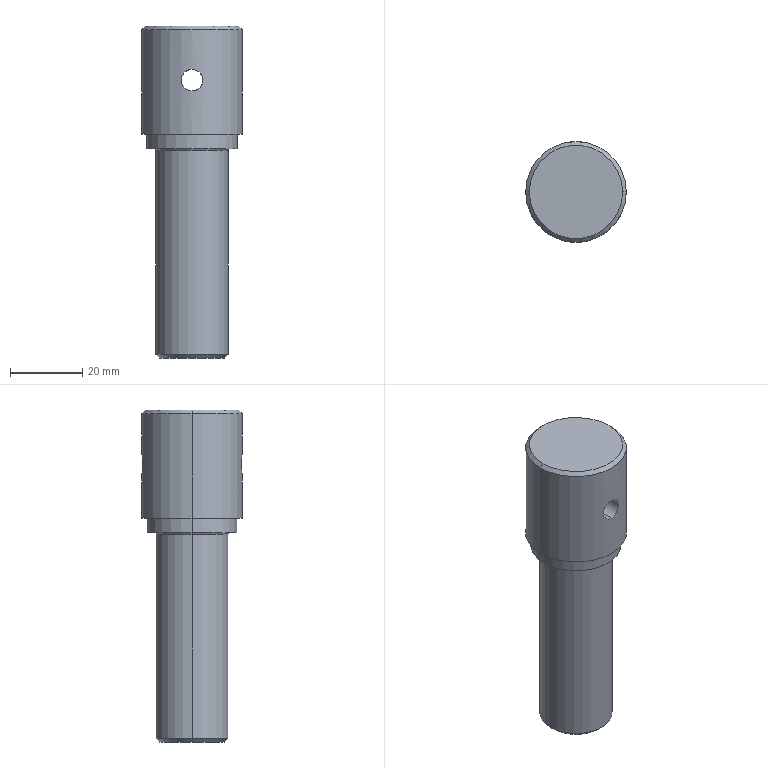Part | SolidWorks | features ICE 3, Chamfer 1, Extrusion 1, Fillet 1 | 1 solid | 18 faces | box 27.9 x 27.9 x 92 mm | volume 37672 mm3 | cylinder 8 | cone 4 | plane 4 | torus 2 | commonest cylinder face diameters 6 x2 20 x2 25 x2 27.9 x2
STEP:
#1=CARTESIAN_POINT('',(0.,-13.95,74.));
#2=VERTEX_POINT('',#1);
#3=CARTESIAN_POINT('',(0.,-13.95,80.));
#4=VERTEX_POINT('',#3);
#5=CARTESIAN_POINT('',(0.,-13.95,74.));
#6=CARTESIAN_POINT('',(-0.3921,-13.95,74.));
#7=CARTESIAN_POINT('',(-0.788,-13.932,74.079));
#8=CARTESIAN_POINT('',(-1.33,-13.888,74.304));
#9=CARTESIAN_POINT('',(-1.505,-13.87,74.397));
#10=CARTESIAN_POINT('',(-1.831,-13.83,74.616));
#11=CARTESIAN_POINT('',(-1.982,-13.809,74.739));
#12=CARTESIAN_POINT('',(-2.259,-13.767,75.016));
#13=CARTESIAN_POINT('',(-2.385,-13.745,75.17));
#14=CARTESIAN_POINT('',(-2.602,-13.706,75.494));
#15=CARTESIAN_POINT('',(-2.694,-13.688,75.666));
#16=CARTESIAN_POINT('',(-2.922,-13.642,76.212));
#17=CARTESIAN_POINT('',(-3.,-13.624,76.603));
#18=CARTESIAN_POINT('',(-3.,-13.624,77.197));
#19=CARTESIAN_POINT('',(-2.981,-13.628,77.392));
#20=CARTESIAN_POINT('',(-2.904,-13.644,77.776));
#21=CARTESIAN_POINT('',(-2.846,-13.657,77.968));
#22=CARTESIAN_POINT('',(-2.696,-13.687,78.33));
#23=CARTESIAN_POINT('',(-2.604,-13.705,78.502));
#24=CARTESIAN_POINT('',(-2.386,-13.745,78.829));
#25=CARTESIAN_POINT('',(-2.26,-13.766,78.982));
#26=CARTESIAN_POINT('',(-1.847,-13.83,79.396));
#27=CARTESIAN_POINT('',(-1.514,-13.872,79.619));
#28=CARTESIAN_POINT('',(-0.9725,-13.917,79.845));
#29=CARTESIAN_POINT('',(-0.7819,-13.929,79.903));
#30=CARTESIAN_POINT('',(-0.3949,-13.946,79.98));
#31=CARTESIAN_POINT('',(-0.1988,-13.95,80.));
#32=CARTESIAN_POINT('',(0.,-13.95,80.));
#33=B_SPLINE_CURVE_WITH_KNOTS('',3,(#5,#6,#7,#8,#9,#10,#11,#12,#13,#14,#15,#16,#17,#18,#19,#20,#21,#22,#23,#24,#25,#26,#27,#28,#29,#30,#31,#32),.UNSPECIFIED.,.F.,.F.,(4,2,2,2,2,2,2,2,2,2,2,2,2,4),(0.009407,0.01058,0.01117,0.01176,0.01235,0.01293,0.01411,0.0147,0.01528,0.01587,0.01646,0.01764,0.01822,0.01881),.UNSPECIFIED.);
#34=EDGE_CURVE('',#2,#4,#33,.T.);
#35=ORIENTED_EDGE('',*,*,#34,.F.);
#36=CARTESIAN_POINT('',(0.,13.95,74.));
#37=VERTEX_POINT('',#36);
#38=CARTESIAN_POINT('',(0.,-15.,74.));
#39=DIRECTION('',(0.,1.,0.));
#40=VECTOR('',#39,1000.);
#41=LINE('',#38,#40);
#42=EDGE_CURVE('',#2,#37,#41,.T.);
#43=ORIENTED_EDGE('',*,*,#42,.T.);
#44=CARTESIAN_POINT('',(0.,13.95,80.));
#45=VERTEX_POINT('',#44);
#46=CARTESIAN_POINT('',(0.,13.95,80.));
#47=CARTESIAN_POINT('',(-0.1988,13.95,80.));
#48=CARTESIAN_POINT('',(-0.3942,13.946,79.98));
#49=CARTESIAN_POINT('',(-0.7785,13.93,79.904));
#50=CARTESIAN_POINT('',(-0.9694,13.917,79.846));
#51=CARTESIAN_POINT('',(-1.332,13.887,79.695));
#52=CARTESIAN_POINT('',(-1.505,13.87,79.603));
#53=CARTESIAN_POINT('',(-1.83,13.83,79.385));
#54=CARTESIAN_POINT('',(-1.984,13.809,79.259));
#55=CARTESIAN_POINT('',(-2.26,13.766,78.983));
#56=CARTESIAN_POINT('',(-2.384,13.745,78.832));
#57=CARTESIAN_POINT('',(-2.603,13.705,78.504));
#58=CARTESIAN_POINT('',(-2.696,13.687,78.331));
#59=CARTESIAN_POINT('',(-2.846,13.657,77.97));
#60=CARTESIAN_POINT('',(-2.904,13.645,77.78));
#61=CARTESIAN_POINT('',(-2.981,13.628,77.393));
#62=CARTESIAN_POINT('',(-3.,13.624,77.198));
#63=CARTESIAN_POINT('',(-3.,13.624,76.805));
#64=CARTESIAN_POINT('',(-2.98,13.628,76.605));
#65=CARTESIAN_POINT('',(-2.904,13.645,76.22));
#66=CARTESIAN_POINT('',(-2.847,13.657,76.033));
#67=CARTESIAN_POINT('',(-2.696,13.687,75.669));
#68=CARTESIAN_POINT('',(-2.602,13.706,75.494));
#69=CARTESIAN_POINT('',(-2.385,13.745,75.17));
#70=CARTESIAN_POINT('',(-2.26,13.766,75.018));
#71=CARTESIAN_POINT('',(-1.982,13.809,74.739));
#72=CARTESIAN_POINT('',(-1.831,13.83,74.615));
#73=CARTESIAN_POINT('',(-1.506,13.869,74.398));
#74=CARTESIAN_POINT('',(-1.331,13.888,74.304));
#75=CARTESIAN_POINT('',(-0.9682,13.918,74.154));
#76=CARTESIAN_POINT('',(-0.7811,13.929,74.097));
#77=CARTESIAN_POINT('',(-0.3953,13.946,74.02));
#78=CARTESIAN_POINT('',(-0.1961,13.95,74.));
#79=CARTESIAN_POINT('',(0.,13.95,74.));
#80=B_SPLINE_CURVE_WITH_KNOTS('',3,(#46,#47,#48,#49,#50,#51,#52,#53,#54,#55,#56,#57,#58,#59,#60,#61,#62,#63,#64,#65,#66,#67,#68,#69,#70,#71,#72,#73,#74,#75,#76,#77,#78,#79),.UNSPECIFIED.,.F.,.F.,(4,2,2,2,2,2,2,2,2,2,2,2,2,2,2,2,4),(0.,0.0005879,0.001176,0.001764,0.002352,0.00294,0.003528,0.004116,0.004703,0.005291,0.005879,0.006467,0.007055,0.007643,0.008231,0.008819,0.009407),.UNSPECIFIED.);
#81=EDGE_CURVE('',#45,#37,#80,.T.);
#82=ORIENTED_EDGE('',*,*,#81,.F.);
#83=CARTESIAN_POINT('',(0.,-15.,80.));
#84=DIRECTION('',(0.,1.,0.));
#85=VECTOR('',#84,1000.);
#86=LINE('',#83,#85);
#87=EDGE_CURVE('',#4,#45,#86,.T.);
#88=ORIENTED_EDGE('',*,*,#87,.F.);
#89=EDGE_LOOP('',(#35,#43,#82,#88));
#90=FACE_OUTER_BOUND('',#89,.T.);
#91=CARTESIAN_POINT('',(0.,-15.,77.));
#92=DIRECTION('',(0.,1.,0.));
#93=DIRECTION('',(0.,0.,1.));
#94=AXIS2_PLACEMENT_3D('',#91,#92,#93);
#95=CYLINDRICAL_SURFACE('',#94,3.);
#96=ADVANCED_FACE('',(#90),#95,.F.);
#97=CARTESIAN_POINT('',(-10.5,0.,58.));
#98=VERTEX_POINT('',#97);
#99=CARTESIAN_POINT('',(10.5,0.,58.));
#100=VERTEX_POINT('',#99);
#101=CARTESIAN_POINT('',(0.,0.,58.));
#102=DIRECTION('',(0.,0.,1.));
#103=DIRECTION('',(1.,0.,0.));
#104=AXIS2_PLACEMENT_3D('',#101,#102,#103);
#105=CIRCLE('',#104,10.5);
#106=EDGE_CURVE('',#98,#100,#105,.T.);
#107=ORIENTED_EDGE('',*,*,#106,.F.);
#108=CARTESIAN_POINT('',(-10.,0.,57.5));
#109=VERTEX_POINT('',#108);
#110=CARTESIAN_POINT('',(-10.5,0.,57.5));
#111=DIRECTION('',(0.,1.,0.));
#112=DIRECTION('',(-1.,0.,0.));
#113=AXIS2_PLACEMENT_3D('',#110,#111,#112);
#114=CIRCLE('',#113,0.5);
#115=EDGE_CURVE('',#98,#109,#114,.T.);
#116=ORIENTED_EDGE('',*,*,#115,.T.);
#117=CARTESIAN_POINT('',(10.,0.,57.5));
#118=VERTEX_POINT('',#117);
#119=CARTESIAN_POINT('',(0.,0.,57.5));
#120=DIRECTION('',(0.,0.,-1.));
#121=DIRECTION('',(1.,0.,0.));
#122=AXIS2_PLACEMENT_3D('',#119,#120,#121);
#123=CIRCLE('',#122,10.);
#124=EDGE_CURVE('',#118,#109,#123,.T.);
#125=ORIENTED_EDGE('',*,*,#124,.F.);
#126=CARTESIAN_POINT('',(10.5,0.,57.5));
#127=DIRECTION('',(0.,-1.,0.));
#128=DIRECTION('',(0.,0.,-1.));
#129=AXIS2_PLACEMENT_3D('',#126,#127,#128);
#130=CIRCLE('',#129,0.5);
#131=EDGE_CURVE('',#100,#118,#130,.T.);
#132=ORIENTED_EDGE('',*,*,#131,.F.);
#133=EDGE_LOOP('',(#107,#116,#125,#132));
#134=FACE_OUTER_BOUND('',#133,.T.);
#135=CARTESIAN_POINT('',(0.,0.,57.5));
#136=DIRECTION('',(0.,0.,1.));
#137=DIRECTION('',(1.,0.,0.));
#138=AXIS2_PLACEMENT_3D('',#135,#136,#137);
#139=TOROIDAL_SURFACE('',#138,10.5,0.5);
#140=ADVANCED_FACE('',(#134),#139,.F.);
#141=CARTESIAN_POINT('',(12.95,0.,92.));
#142=VERTEX_POINT('',#141);
#143=CARTESIAN_POINT('',(-12.95,0.,92.));
#144=VERTEX_POINT('',#143);
#145=CARTESIAN_POINT('',(0.,0.,92.));
#146=DIRECTION('',(0.,0.,1.));
#147=DIRECTION('',(1.,0.,0.));
#148=AXIS2_PLACEMENT_3D('',#145,#146,#147);
#149=CIRCLE('',#148,12.95);
#150=EDGE_CURVE('',#142,#144,#149,.T.);
#151=ORIENTED_EDGE('',*,*,#150,.F.);
#152=CARTESIAN_POINT('',(13.95,0.,91.));
#153=VERTEX_POINT('',#152);
#154=CARTESIAN_POINT('',(12.95,0.,92.));
#155=DIRECTION('',(0.7071,0.,-0.7071));
#156=VECTOR('',#155,1000.);
#157=LINE('',#154,#156);
#158=EDGE_CURVE('',#142,#153,#157,.T.);
#159=ORIENTED_EDGE('',*,*,#158,.T.);
#160=CARTESIAN_POINT('',(-13.95,0.,91.));
#161=VERTEX_POINT('',#160);
#162=CARTESIAN_POINT('',(0.,0.,91.));
#163=DIRECTION('',(0.,0.,-1.));
#164=DIRECTION('',(1.,0.,0.));
#165=AXIS2_PLACEMENT_3D('',#162,#163,#164);
#166=CIRCLE('',#165,13.95);
#167=EDGE_CURVE('',#161,#153,#166,.T.);
#168=ORIENTED_EDGE('',*,*,#167,.F.);
#169=CARTESIAN_POINT('',(-12.95,0.,92.));
#170=DIRECTION('',(-0.7071,0.,-0.7071));
#171=VECTOR('',#170,1000.);
#172=LINE('',#169,#171);
#173=EDGE_CURVE('',#144,#161,#172,.T.);
#174=ORIENTED_EDGE('',*,*,#173,.F.);
#175=EDGE_LOOP('',(#151,#159,#168,#174));
#176=FACE_OUTER_BOUND('',#175,.T.);
#177=CARTESIAN_POINT('',(0.,0.,92.));
#178=DIRECTION('',(0.,0.,-1.));
#179=DIRECTION('',(-1.,0.,0.));
#180=AXIS2_PLACEMENT_3D('',#177,#178,#179);
#181=CONICAL_SURFACE('',#180,12.95,0.7854);
#182=ADVANCED_FACE('',(#176),#181,.T.);
#183=CARTESIAN_POINT('',(-9.,0.,0.));
#184=VERTEX_POINT('',#183);
#185=CARTESIAN_POINT('',(9.,0.,0.));
#186=VERTEX_POINT('',#185);
#187=CARTESIAN_POINT('',(0.,0.,0.));
#188=DIRECTION('',(0.,0.,-1.));
#189=DIRECTION('',(1.,0.,0.));
#190=AXIS2_PLACEMENT_3D('',#187,#188,#189);
#191=CIRCLE('',#190,9.);
#192=EDGE_CURVE('',#184,#186,#191,.T.);
#193=ORIENTED_EDGE('',*,*,#192,.F.);
#194=CARTESIAN_POINT('',(-10.,0.,1.));
#195=VERTEX_POINT('',#194);
#196=CARTESIAN_POINT('',(-10.,0.,1.));
#197=DIRECTION('',(-0.7071,0.,0.7071));
#198=VECTOR('',#197,1000.);
#199=LINE('',#196,#198);
#200=EDGE_CURVE('',#184,#195,#199,.T.);
#201=ORIENTED_EDGE('',*,*,#200,.T.);
#202=CARTESIAN_POINT('',(10.,0.,1.));
#203=VERTEX_POINT('',#202);
#204=CARTESIAN_POINT('',(0.,0.,1.));
#205=DIRECTION('',(0.,0.,1.));
#206=DIRECTION('',(1.,0.,0.));
#207=AXIS2_PLACEMENT_3D('',#204,#205,#206);
#208=CIRCLE('',#207,10.);
#209=EDGE_CURVE('',#203,#195,#208,.T.);
#210=ORIENTED_EDGE('',*,*,#209,.F.);
#211=CARTESIAN_POINT('',(10.,0.,1.));
#212=DIRECTION('',(0.7071,0.,0.7071));
#213=VECTOR('',#212,1000.);
#214=LINE('',#211,#213);
#215=EDGE_CURVE('',#186,#203,#214,.T.);
#216=ORIENTED_EDGE('',*,*,#215,.F.);
#217=EDGE_LOOP('',(#193,#201,#210,#216));
#218=FACE_OUTER_BOUND('',#217,.T.);
#219=CARTESIAN_POINT('',(0.,0.,1.));
#220=DIRECTION('',(0.,0.,1.));
#221=DIRECTION('',(1.,0.,0.));
#222=AXIS2_PLACEMENT_3D('',#219,#220,#221);
#223=CONICAL_SURFACE('',#222,10.,0.7854);
#224=ADVANCED_FACE('',(#218),#223,.T.);
#225=ORIENTED_EDGE('',*,*,#81,.T.);
#226=CARTESIAN_POINT('',(0.,13.95,74.));
#227=CARTESIAN_POINT('',(0.3921,13.95,74.));
#228=CARTESIAN_POINT('',(0.788,13.932,74.079));
#229=CARTESIAN_POINT('',(1.33,13.888,74.304));
#230=CARTESIAN_POINT('',(1.505,13.87,74.397));
#231=CARTESIAN_POINT('',(1.831,13.83,74.616));
#232=CARTESIAN_POINT('',(1.982,13.809,74.739));
#233=CARTESIAN_POINT('',(2.259,13.767,75.016));
#234=CARTESIAN_POINT('',(2.385,13.745,75.17));
#235=CARTESIAN_POINT('',(2.602,13.706,75.494));
#236=CARTESIAN_POINT('',(2.694,13.688,75.666));
#237=CARTESIAN_POINT('',(2.922,13.642,76.212));
#238=CARTESIAN_POINT('',(3.,13.624,76.603));
#239=CARTESIAN_POINT('',(3.,13.624,77.197));
#240=CARTESIAN_POINT('',(2.981,13.628,77.392));
#241=CARTESIAN_POINT('',(2.904,13.644,77.776));
#242=CARTESIAN_POINT('',(2.846,13.657,77.968));
#243=CARTESIAN_POINT('',(2.696,13.687,78.33));
#244=CARTESIAN_POINT('',(2.604,13.705,78.502));
#245=CARTESIAN_POINT('',(2.386,13.745,78.829));
#246=CARTESIAN_POINT('',(2.26,13.766,78.982));
#247=CARTESIAN_POINT('',(1.847,13.83,79.396));
#248=CARTESIAN_POINT('',(1.514,13.872,79.619));
#249=CARTESIAN_POINT('',(0.9725,13.917,79.845));
#250=CARTESIAN_POINT('',(0.7819,13.929,79.903));
#251=CARTESIAN_POINT('',(0.3949,13.946,79.98));
#252=CARTESIAN_POINT('',(0.1988,13.95,80.));
#253=CARTESIAN_POINT('',(0.,13.95,80.));
#254=B_SPLINE_CURVE_WITH_KNOTS('',3,(#226,#227,#228,#229,#230,#231,#232,#233,#234,#235,#236,#237,#238,#239,#240,#241,#242,#243,#244,#245,#246,#247,#248,#249,#250,#251,#252,#253),.UNSPECIFIED.,.F.,.F.,(4,2,2,2,2,2,2,2,2,2,2,2,2,4),(0.009407,0.01058,0.01117,0.01176,0.01235,0.01293,0.01411,0.0147,0.01528,0.01587,0.01646,0.01764,0.01822,0.01881),.UNSPECIFIED.);
#255=EDGE_CURVE('',#37,#45,#254,.T.);
#256=ORIENTED_EDGE('',*,*,#255,.T.);
#257=EDGE_LOOP('',(#225,#256));
#258=FACE_BOUND('',#257,.T.);
#259=ORIENTED_EDGE('',*,*,#167,.T.);
#260=CARTESIAN_POINT('',(13.95,0.,62.));
#261=VERTEX_POINT('',#260);
#262=CARTESIAN_POINT('',(13.95,0.,92.));
#263=DIRECTION('',(0.,0.,-1.));
#264=VECTOR('',#263,1000.);
#265=LINE('',#262,#264);
#266=EDGE_CURVE('',#153,#261,#265,.T.);
#267=ORIENTED_EDGE('',*,*,#266,.T.);
#268=CARTESIAN_POINT('',(-13.95,0.,62.));
#269=VERTEX_POINT('',#268);
#270=CARTESIAN_POINT('',(0.,0.,62.));
#271=DIRECTION('',(0.,0.,1.));
#272=DIRECTION('',(1.,0.,0.));
#273=AXIS2_PLACEMENT_3D('',#270,#271,#272);
#274=CIRCLE('',#273,13.95);
#275=EDGE_CURVE('',#261,#269,#274,.T.);
#276=ORIENTED_EDGE('',*,*,#275,.T.);
#277=CARTESIAN_POINT('',(-13.95,0.,92.));
#278=DIRECTION('',(0.,0.,-1.));
#279=VECTOR('',#278,1000.);
#280=LINE('',#277,#279);
#281=EDGE_CURVE('',#161,#269,#280,.T.);
#282=ORIENTED_EDGE('',*,*,#281,.F.);
#283=EDGE_LOOP('',(#259,#267,#276,#282));
#284=FACE_OUTER_BOUND('',#283,.T.);
#285=CARTESIAN_POINT('',(0.,0.,92.));
#286=DIRECTION('',(0.,0.,-1.));
#287=DIRECTION('',(-1.,0.,0.));
#288=AXIS2_PLACEMENT_3D('',#285,#286,#287);
#289=CYLINDRICAL_SURFACE('',#288,13.95);
#290=ADVANCED_FACE('',(#258,#284),#289,.T.);
#291=CARTESIAN_POINT('',(12.5,0.,62.));
#292=VERTEX_POINT('',#291);
#293=CARTESIAN_POINT('',(-12.5,0.,62.));
#294=VERTEX_POINT('',#293);
#295=CARTESIAN_POINT('',(0.,0.,62.));
#296=DIRECTION('',(0.,0.,1.));
#297=DIRECTION('',(1.,0.,0.));
#298=AXIS2_PLACEMENT_3D('',#295,#296,#297);
#299=CIRCLE('',#298,12.5);
#300=EDGE_CURVE('',#292,#294,#299,.T.);
#301=ORIENTED_EDGE('',*,*,#300,.F.);
#302=CARTESIAN_POINT('',(12.5,0.,58.));
#303=VERTEX_POINT('',#302);
#304=CARTESIAN_POINT('',(12.5,0.,62.));
#305=DIRECTION('',(0.,0.,-1.));
#306=VECTOR('',#305,1000.);
#307=LINE('',#304,#306);
#308=EDGE_CURVE('',#292,#303,#307,.T.);
#309=ORIENTED_EDGE('',*,*,#308,.T.);
#310=CARTESIAN_POINT('',(-12.5,0.,58.));
#311=VERTEX_POINT('',#310);
#312=CARTESIAN_POINT('',(0.,0.,58.));
#313=DIRECTION('',(0.,0.,1.));
#314=DIRECTION('',(1.,0.,0.));
#315=AXIS2_PLACEMENT_3D('',#312,#313,#314);
#316=CIRCLE('',#315,12.5);
#317=EDGE_CURVE('',#303,#311,#316,.T.);
#318=ORIENTED_EDGE('',*,*,#317,.T.);
#319=CARTESIAN_POINT('',(-12.5,0.,62.));
#320=DIRECTION('',(0.,0.,-1.));
#321=VECTOR('',#320,1000.);
#322=LINE('',#319,#321);
#323=EDGE_CURVE('',#294,#311,#322,.T.);
#324=ORIENTED_EDGE('',*,*,#323,.F.);
#325=EDGE_LOOP('',(#301,#309,#318,#324));
#326=FACE_OUTER_BOUND('',#325,.T.);
#327=CARTESIAN_POINT('',(0.,0.,62.));
#328=DIRECTION('',(0.,0.,-1.));
#329=DIRECTION('',(-1.,0.,0.));
#330=AXIS2_PLACEMENT_3D('',#327,#328,#329);
#331=CYLINDRICAL_SURFACE('',#330,12.5);
#332=ADVANCED_FACE('',(#326),#331,.T.);
#333=CARTESIAN_POINT('',(0.,0.,57.5));
#334=DIRECTION('',(0.,0.,-1.));
#335=DIRECTION('',(1.,0.,0.));
#336=AXIS2_PLACEMENT_3D('',#333,#334,#335);
#337=CIRCLE('',#336,10.);
#338=EDGE_CURVE('',#109,#118,#337,.T.);
#339=ORIENTED_EDGE('',*,*,#338,.T.);
#340=CARTESIAN_POINT('',(10.,0.,58.));
#341=DIRECTION('',(0.,0.,-1.));
#342=VECTOR('',#341,1000.);
#343=LINE('',#340,#342);
#344=EDGE_CURVE('',#118,#203,#343,.T.);
#345=ORIENTED_EDGE('',*,*,#344,.T.);
#346=ORIENTED_EDGE('',*,*,#209,.T.);
#347=CARTESIAN_POINT('',(-10.,0.,58.));
#348=DIRECTION('',(0.,0.,-1.));
#349=VECTOR('',#348,1000.);
#350=LINE('',#347,#349);
#351=EDGE_CURVE('',#109,#195,#350,.T.);
#352=ORIENTED_EDGE('',*,*,#351,.F.);
#353=EDGE_LOOP('',(#339,#345,#346,#352));
#354=FACE_OUTER_BOUND('',#353,.T.);
#355=CARTESIAN_POINT('',(0.,0.,58.));
#356=DIRECTION('',(0.,0.,-1.));
#357=DIRECTION('',(-1.,0.,0.));
#358=AXIS2_PLACEMENT_3D('',#355,#356,#357);
#359=CYLINDRICAL_SURFACE('',#358,10.);
#360=ADVANCED_FACE('',(#354),#359,.T.);
#361=ORIENTED_EDGE('',*,*,#344,.F.);
#362=ORIENTED_EDGE('',*,*,#124,.T.);
#363=ORIENTED_EDGE('',*,*,#351,.T.);
#364=CARTESIAN_POINT('',(0.,0.,1.));
#365=DIRECTION('',(0.,0.,1.));
#366=DIRECTION('',(1.,0.,0.));
#367=AXIS2_PLACEMENT_3D('',#364,#365,#366);
#368=CIRCLE('',#367,10.);
#369=EDGE_CURVE('',#195,#203,#368,.T.);
#370=ORIENTED_EDGE('',*,*,#369,.T.);
#371=EDGE_LOOP('',(#361,#362,#363,#370));
#372=FACE_OUTER_BOUND('',#371,.T.);
#373=CARTESIAN_POINT('',(0.,0.,58.));
#374=DIRECTION('',(0.,0.,-1.));
#375=DIRECTION('',(-1.,0.,0.));
#376=AXIS2_PLACEMENT_3D('',#373,#374,#375);
#377=CYLINDRICAL_SURFACE('',#376,10.);
#378=ADVANCED_FACE('',(#372),#377,.T.);
#379=CARTESIAN_POINT('',(0.,0.,0.));
#380=DIRECTION('',(0.,0.,-1.));
#381=DIRECTION('',(1.,0.,0.));
#382=AXIS2_PLACEMENT_3D('',#379,#380,#381);
#383=CIRCLE('',#382,9.);
#384=EDGE_CURVE('',#186,#184,#383,.T.);
#385=ORIENTED_EDGE('',*,*,#384,.T.);
#386=ORIENTED_EDGE('',*,*,#192,.T.);
#387=EDGE_LOOP('',(#385,#386));
#388=FACE_OUTER_BOUND('',#387,.T.);
#389=CARTESIAN_POINT('',(0.,0.,0.));
#390=DIRECTION('',(0.,0.,1.));
#391=DIRECTION('',(1.,0.,0.));
#392=AXIS2_PLACEMENT_3D('',#389,#390,#391);
#393=PLANE('',#392);
#394=ADVANCED_FACE('',(#388),#393,.F.);
#395=ORIENTED_EDGE('',*,*,#308,.F.);
#396=CARTESIAN_POINT('',(0.,0.,62.));
#397=DIRECTION('',(0.,0.,1.));
#398=DIRECTION('',(1.,0.,0.));
#399=AXIS2_PLACEMENT_3D('',#396,#397,#398);
#400=CIRCLE('',#399,12.5);
#401=EDGE_CURVE('',#294,#292,#400,.T.);
#402=ORIENTED_EDGE('',*,*,#401,.F.);
#403=ORIENTED_EDGE('',*,*,#323,.T.);
#404=CARTESIAN_POINT('',(0.,0.,58.));
#405=DIRECTION('',(0.,0.,1.));
#406=DIRECTION('',(1.,0.,0.));
#407=AXIS2_PLACEMENT_3D('',#404,#405,#406);
#408=CIRCLE('',#407,12.5);
#409=EDGE_CURVE('',#311,#303,#408,.T.);
#410=ORIENTED_EDGE('',*,*,#409,.T.);
#411=EDGE_LOOP('',(#395,#402,#403,#410));
#412=FACE_OUTER_BOUND('',#411,.T.);
#413=CARTESIAN_POINT('',(0.,0.,62.));
#414=DIRECTION('',(0.,0.,-1.));
#415=DIRECTION('',(-1.,0.,0.));
#416=AXIS2_PLACEMENT_3D('',#413,#414,#415);
#417=CYLINDRICAL_SURFACE('',#416,12.5);
#418=ADVANCED_FACE('',(#412),#417,.T.);
#419=CARTESIAN_POINT('',(0.,0.,58.));
#420=DIRECTION('',(0.,0.,1.));
#421=DIRECTION('',(1.,0.,0.));
#422=AXIS2_PLACEMENT_3D('',#419,#420,#421);
#423=CIRCLE('',#422,10.5);
#424=EDGE_CURVE('',#100,#98,#423,.T.);
#425=ORIENTED_EDGE('',*,*,#424,.T.);
#426=ORIENTED_EDGE('',*,*,#106,.T.);
#427=EDGE_LOOP('',(#425,#426));
#428=FACE_BOUND('',#427,.T.);
#429=ORIENTED_EDGE('',*,*,#409,.F.);
#430=ORIENTED_EDGE('',*,*,#317,.F.);
#431=EDGE_LOOP('',(#429,#430));
#432=FACE_OUTER_BOUND('',#431,.T.);
#433=CARTESIAN_POINT('',(0.,0.,58.));
#434=DIRECTION('',(0.,0.,1.));
#435=DIRECTION('',(1.,0.,0.));
#436=AXIS2_PLACEMENT_3D('',#433,#434,#435);
#437=PLANE('',#436);
#438=ADVANCED_FACE('',(#428,#432),#437,.F.);
#439=ORIENTED_EDGE('',*,*,#266,.F.);
#440=CARTESIAN_POINT('',(0.,0.,91.));
#441=DIRECTION('',(0.,0.,-1.));
#442=DIRECTION('',(1.,0.,0.));
#443=AXIS2_PLACEMENT_3D('',#440,#441,#442);
#444=CIRCLE('',#443,13.95);
#445=EDGE_CURVE('',#153,#161,#444,.T.);
#446=ORIENTED_EDGE('',*,*,#445,.T.);
#447=ORIENTED_EDGE('',*,*,#281,.T.);
#448=CARTESIAN_POINT('',(0.,0.,62.));
#449=DIRECTION('',(0.,0.,1.));
#450=DIRECTION('',(1.,0.,0.));
#451=AXIS2_PLACEMENT_3D('',#448,#449,#450);
#452=CIRCLE('',#451,13.95);
#453=EDGE_CURVE('',#269,#261,#452,.T.);
#454=ORIENTED_EDGE('',*,*,#453,.T.);
#455=EDGE_LOOP('',(#439,#446,#447,#454));
#456=FACE_OUTER_BOUND('',#455,.T.);
#457=CARTESIAN_POINT('',(0.,-13.95,80.));
#458=CARTESIAN_POINT('',(0.1988,-13.95,80.));
#459=CARTESIAN_POINT('',(0.3942,-13.946,79.98));
#460=CARTESIAN_POINT('',(0.7785,-13.93,79.904));
#461=CARTESIAN_POINT('',(0.9694,-13.917,79.846));
#462=CARTESIAN_POINT('',(1.332,-13.887,79.695));
#463=CARTESIAN_POINT('',(1.505,-13.87,79.603));
#464=CARTESIAN_POINT('',(1.83,-13.83,79.385));
#465=CARTESIAN_POINT('',(1.984,-13.809,79.259));
#466=CARTESIAN_POINT('',(2.26,-13.766,78.983));
#467=CARTESIAN_POINT('',(2.384,-13.745,78.832));
#468=CARTESIAN_POINT('',(2.603,-13.705,78.504));
#469=CARTESIAN_POINT('',(2.696,-13.687,78.331));
#470=CARTESIAN_POINT('',(2.846,-13.657,77.97));
#471=CARTESIAN_POINT('',(2.904,-13.645,77.78));
#472=CARTESIAN_POINT('',(2.981,-13.628,77.393));
#473=CARTESIAN_POINT('',(3.,-13.624,77.198));
#474=CARTESIAN_POINT('',(3.,-13.624,76.805));
#475=CARTESIAN_POINT('',(2.98,-13.628,76.605));
#476=CARTESIAN_POINT('',(2.904,-13.645,76.22));
#477=CARTESIAN_POINT('',(2.847,-13.657,76.033));
#478=CARTESIAN_POINT('',(2.696,-13.687,75.669));
#479=CARTESIAN_POINT('',(2.602,-13.706,75.494));
#480=CARTESIAN_POINT('',(2.385,-13.745,75.17));
#481=CARTESIAN_POINT('',(2.26,-13.766,75.018));
#482=CARTESIAN_POINT('',(1.982,-13.809,74.739));
#483=CARTESIAN_POINT('',(1.831,-13.83,74.615));
#484=CARTESIAN_POINT('',(1.506,-13.869,74.398));
#485=CARTESIAN_POINT('',(1.331,-13.888,74.304));
#486=CARTESIAN_POINT('',(0.9682,-13.918,74.154));
#487=CARTESIAN_POINT('',(0.7811,-13.929,74.097));
#488=CARTESIAN_POINT('',(0.3953,-13.946,74.02));
#489=CARTESIAN_POINT('',(0.1961,-13.95,74.));
#490=CARTESIAN_POINT('',(0.,-13.95,74.));
#491=B_SPLINE_CURVE_WITH_KNOTS('',3,(#457,#458,#459,#460,#461,#462,#463,#464,#465,#466,#467,#468,#469,#470,#471,#472,#473,#474,#475,#476,#477,#478,#479,#480,#481,#482,#483,#484,#485,#486,#487,#488,#489,#490),.UNSPECIFIED.,.F.,.F.,(4,2,2,2,2,2,2,2,2,2,2,2,2,2,2,2,4),(0.,0.0005879,0.001176,0.001764,0.002352,0.00294,0.003528,0.004116,0.004703,0.005291,0.005879,0.006467,0.007055,0.007643,0.008231,0.008819,0.009407),.UNSPECIFIED.);
#492=EDGE_CURVE('',#4,#2,#491,.T.);
#493=ORIENTED_EDGE('',*,*,#492,.T.);
#494=ORIENTED_EDGE('',*,*,#34,.T.);
#495=EDGE_LOOP('',(#493,#494));
#496=FACE_BOUND('',#495,.T.);
#497=CARTESIAN_POINT('',(0.,0.,92.));
#498=DIRECTION('',(0.,0.,-1.));
#499=DIRECTION('',(-1.,0.,0.));
#500=AXIS2_PLACEMENT_3D('',#497,#498,#499);
#501=CYLINDRICAL_SURFACE('',#500,13.95);
#502=ADVANCED_FACE('',(#456,#496),#501,.T.);
#503=CARTESIAN_POINT('',(0.,0.,92.));
#504=DIRECTION('',(0.,0.,1.));
#505=DIRECTION('',(1.,0.,0.));
#506=AXIS2_PLACEMENT_3D('',#503,#504,#505);
#507=CIRCLE('',#506,12.95);
#508=EDGE_CURVE('',#144,#142,#507,.T.);
#509=ORIENTED_EDGE('',*,*,#508,.T.);
#510=ORIENTED_EDGE('',*,*,#150,.T.);
#511=EDGE_LOOP('',(#509,#510));
#512=FACE_OUTER_BOUND('',#511,.T.);
#513=CARTESIAN_POINT('',(0.,0.,92.));
#514=DIRECTION('',(0.,0.,1.));
#515=DIRECTION('',(1.,0.,0.));
#516=AXIS2_PLACEMENT_3D('',#513,#514,#515);
#517=PLANE('',#516);
#518=ADVANCED_FACE('',(#512),#517,.T.);
#519=ORIENTED_EDGE('',*,*,#401,.T.);
#520=ORIENTED_EDGE('',*,*,#300,.T.);
#521=EDGE_LOOP('',(#519,#520));
#522=FACE_BOUND('',#521,.T.);
#523=ORIENTED_EDGE('',*,*,#453,.F.);
#524=ORIENTED_EDGE('',*,*,#275,.F.);
#525=EDGE_LOOP('',(#523,#524));
#526=FACE_OUTER_BOUND('',#525,.T.);
#527=CARTESIAN_POINT('',(0.,0.,62.));
#528=DIRECTION('',(0.,0.,1.));
#529=DIRECTION('',(1.,0.,0.));
#530=AXIS2_PLACEMENT_3D('',#527,#528,#529);
#531=PLANE('',#530);
#532=ADVANCED_FACE('',(#522,#526),#531,.F.);
#533=ORIENTED_EDGE('',*,*,#200,.F.);
#534=ORIENTED_EDGE('',*,*,#384,.F.);
#535=ORIENTED_EDGE('',*,*,#215,.T.);
#536=ORIENTED_EDGE('',*,*,#369,.F.);
#537=EDGE_LOOP('',(#533,#534,#535,#536));
#538=FACE_OUTER_BOUND('',#537,.T.);
#539=CARTESIAN_POINT('',(0.,0.,1.));
#540=DIRECTION('',(0.,0.,1.));
#541=DIRECTION('',(1.,0.,0.));
#542=AXIS2_PLACEMENT_3D('',#539,#540,#541);
#543=CONICAL_SURFACE('',#542,10.,0.7854);
#544=ADVANCED_FACE('',(#538),#543,.T.);
#545=ORIENTED_EDGE('',*,*,#158,.F.);
#546=ORIENTED_EDGE('',*,*,#508,.F.);
#547=ORIENTED_EDGE('',*,*,#173,.T.);
#548=ORIENTED_EDGE('',*,*,#445,.F.);
#549=EDGE_LOOP('',(#545,#546,#547,#548));
#550=FACE_OUTER_BOUND('',#549,.T.);
#551=CARTESIAN_POINT('',(0.,0.,92.));
#552=DIRECTION('',(0.,0.,-1.));
#553=DIRECTION('',(-1.,0.,0.));
#554=AXIS2_PLACEMENT_3D('',#551,#552,#553);
#555=CONICAL_SURFACE('',#554,12.95,0.7854);
#556=ADVANCED_FACE('',(#550),#555,.T.);
#557=ORIENTED_EDGE('',*,*,#115,.F.);
#558=ORIENTED_EDGE('',*,*,#424,.F.);
#559=ORIENTED_EDGE('',*,*,#131,.T.);
#560=ORIENTED_EDGE('',*,*,#338,.F.);
#561=EDGE_LOOP('',(#557,#558,#559,#560));
#562=FACE_OUTER_BOUND('',#561,.T.);
#563=CARTESIAN_POINT('',(0.,0.,57.5));
#564=DIRECTION('',(0.,0.,1.));
#565=DIRECTION('',(1.,0.,0.));
#566=AXIS2_PLACEMENT_3D('',#563,#564,#565);
#567=TOROIDAL_SURFACE('',#566,10.5,0.5);
#568=ADVANCED_FACE('',(#562),#567,.F.);
#569=ORIENTED_EDGE('',*,*,#42,.F.);
#570=ORIENTED_EDGE('',*,*,#492,.F.);
#571=ORIENTED_EDGE('',*,*,#87,.T.);
#572=ORIENTED_EDGE('',*,*,#255,.F.);
#573=EDGE_LOOP('',(#569,#570,#571,#572));
#574=FACE_OUTER_BOUND('',#573,.T.);
#575=CARTESIAN_POINT('',(0.,-15.,77.));
#576=DIRECTION('',(0.,1.,0.));
#577=DIRECTION('',(0.,0.,1.));
#578=AXIS2_PLACEMENT_3D('',#575,#576,#577);
#579=CYLINDRICAL_SURFACE('',#578,3.);
#580=ADVANCED_FACE('',(#574),#579,.F.);
#581=CLOSED_SHELL('',(#96,#140,#182,#224,#290,#332,#360,#378,#394,#418,#438,#502,#518,#532,#544,#556,#568,#580));
#582=MANIFOLD_SOLID_BREP('',#581);
#583=CARTESIAN_POINT('',(0.,0.,0.));
#584=DIRECTION('',(0.,0.,1.));
#585=DIRECTION('',(1.,0.,0.));
#586=AXIS2_PLACEMENT_3D('',#583,#584,#585);
#587=(LENGTH_UNIT()NAMED_UNIT(*)SI_UNIT(.MILLI.,.METRE.));
#588=UNCERTAINTY_MEASURE_WITH_UNIT(LENGTH_MEASURE(0.00001),#587,'','');
#589=(NAMED_UNIT(*)PLANE_ANGLE_UNIT()SI_UNIT($,.RADIAN.));
#590=(NAMED_UNIT(*)SI_UNIT($,.STERADIAN.)SOLID_ANGLE_UNIT());
#591=(GEOMETRIC_REPRESENTATION_CONTEXT(3)GLOBAL_UNCERTAINTY_ASSIGNED_CONTEXT((#588))GLOBAL_UNIT_ASSIGNED_CONTEXT((#587,#589,#590))REPRESENTATION_CONTEXT('',''));
#592=ADVANCED_BREP_SHAPE_REPRESENTATION('',(#582,#586),#591);